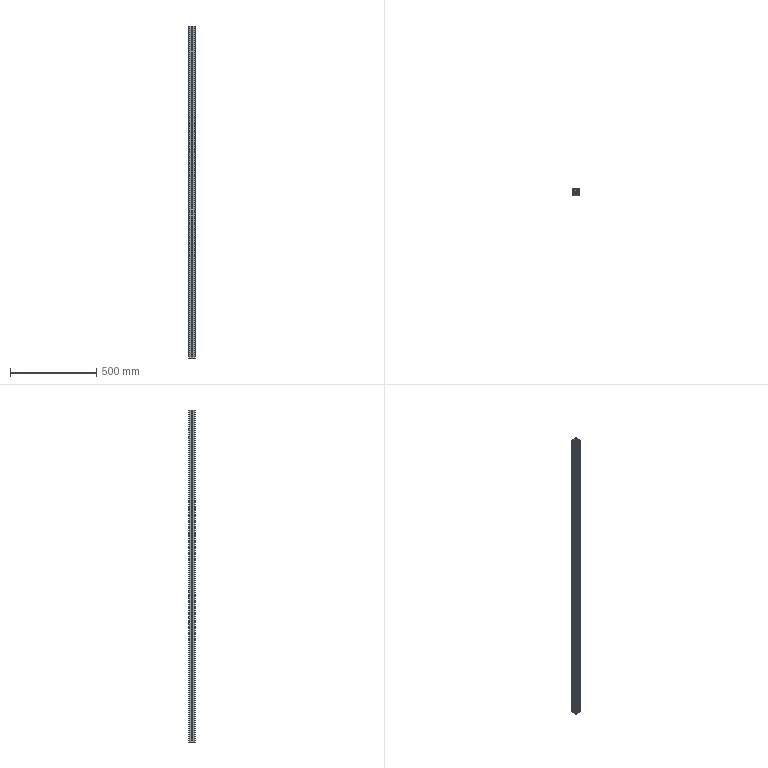Part | SolidWorks | features HoleWzd 4, MoveFace 2, BaseBody 1 | 1 solid | 280 faces | box 40 x 40 x 1930 mm | volume 1139883 mm3 | plane 161 | cylinder 119 | commonest cylinder face diameters 6.8 x47 5 x40 6.6 x8 11 x8 1 x6 2 x6